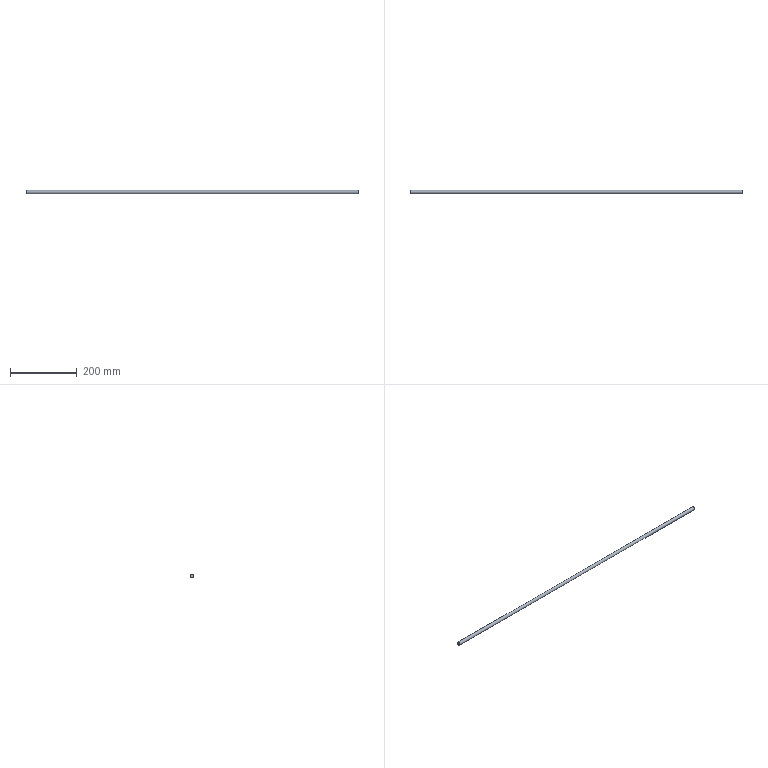Part | STEP file | solid 270 | 1 solid | 3 faces | box 995 x 10 x 10 mm | volume 78147 mm3 | plane 2 | cylinder 1 | commonest cylinder face diameters 10 x1